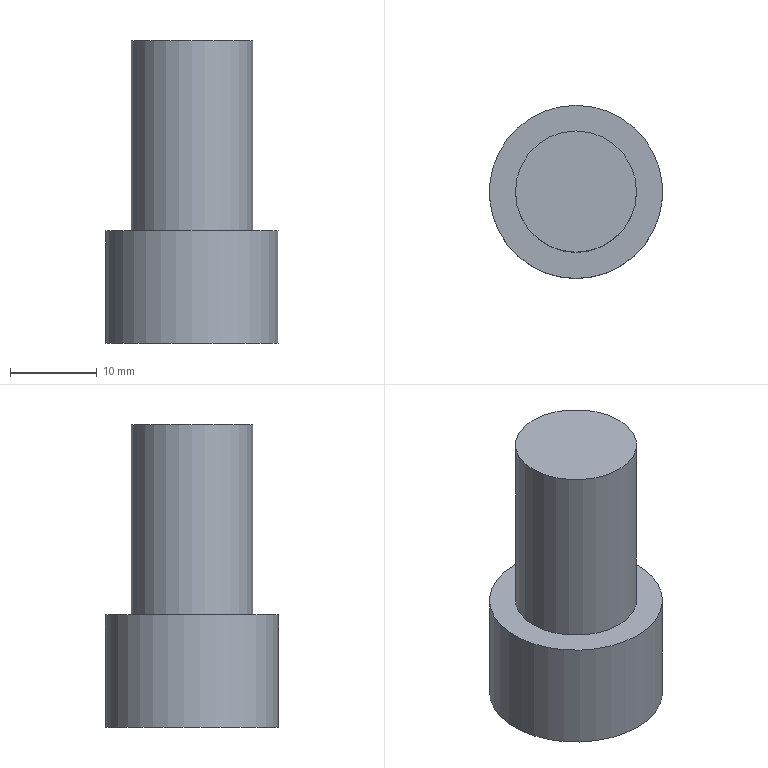Part | NX | features 模具.stp<1>[117] 2 | 1 solid | 5 faces | box 20 x 20 x 35 mm | volume 7471 mm3 | plane 3 | cylinder 2 | commonest cylinder face diameters 14 x1 20 x1
STEP:
#1=CARTESIAN_POINT('',(70.,110.,-285.5));
#2=VERTEX_POINT('',#1);
#3=CARTESIAN_POINT('',(70.,100.,-285.5));
#4=DIRECTION('',(0.,0.,1.));
#5=DIRECTION('',(0.,1.,0.));
#6=AXIS2_PLACEMENT_3D('',#3,#4,#5);
#7=CIRCLE('',#6,10.);
#8=EDGE_CURVE('',#2,#2,#7,.T.);
#9=ORIENTED_EDGE('',*,*,#8,.F.);
#10=EDGE_LOOP('',(#9));
#11=FACE_BOUND('',#10,.T.);
#12=CARTESIAN_POINT('',(70.,100.,-285.5));
#13=DIRECTION('',(0.,0.,-1.));
#14=DIRECTION('',(0.,-1.,0.));
#15=AXIS2_PLACEMENT_3D('',#12,#13,#14);
#16=PLANE('',#15);
#17=ADVANCED_FACE('',(#11),#16,.T.);
#18=CARTESIAN_POINT('',(70.,110.,-272.5));
#19=VERTEX_POINT('',#18);
#20=CARTESIAN_POINT('',(70.,100.,-272.5));
#21=DIRECTION('',(0.,0.,-1.));
#22=DIRECTION('',(0.,1.,0.));
#23=AXIS2_PLACEMENT_3D('',#20,#21,#22);
#24=CIRCLE('',#23,10.);
#25=EDGE_CURVE('',#19,#19,#24,.T.);
#26=ORIENTED_EDGE('',*,*,#25,.T.);
#27=EDGE_LOOP('',(#26));
#28=FACE_BOUND('',#27,.T.);
#29=ORIENTED_EDGE('',*,*,#8,.T.);
#30=EDGE_LOOP('',(#29));
#31=FACE_BOUND('',#30,.T.);
#32=CARTESIAN_POINT('',(70.,100.,-272.5));
#33=DIRECTION('',(0.,0.,-1.));
#34=DIRECTION('',(0.,1.,0.));
#35=AXIS2_PLACEMENT_3D('',#32,#33,#34);
#36=CYLINDRICAL_SURFACE('',#35,10.);
#37=ADVANCED_FACE('',(#28,#31),#36,.T.);
#38=ORIENTED_EDGE('',*,*,#25,.F.);
#39=EDGE_LOOP('',(#38));
#40=FACE_BOUND('',#39,.T.);
#41=CARTESIAN_POINT('',(70.,93.,-272.5));
#42=VERTEX_POINT('',#41);
#43=CARTESIAN_POINT('',(70.,100.,-272.5));
#44=DIRECTION('',(0.,0.,-1.));
#45=DIRECTION('',(0.,-1.,0.));
#46=AXIS2_PLACEMENT_3D('',#43,#44,#45);
#47=CIRCLE('',#46,7.);
#48=EDGE_CURVE('',#42,#42,#47,.T.);
#49=ORIENTED_EDGE('',*,*,#48,.T.);
#50=EDGE_LOOP('',(#49));
#51=FACE_BOUND('',#50,.T.);
#52=CARTESIAN_POINT('',(70.,100.,-272.5));
#53=DIRECTION('',(0.,0.,1.));
#54=DIRECTION('',(0.,-1.,0.));
#55=AXIS2_PLACEMENT_3D('',#52,#53,#54);
#56=PLANE('',#55);
#57=ADVANCED_FACE('',(#40,#51),#56,.T.);
#58=CARTESIAN_POINT('',(70.,107.,-250.5));
#59=VERTEX_POINT('',#58);
#60=CARTESIAN_POINT('',(70.,100.,-250.5));
#61=DIRECTION('',(0.,0.,-1.));
#62=DIRECTION('',(0.,1.,0.));
#63=AXIS2_PLACEMENT_3D('',#60,#61,#62);
#64=CIRCLE('',#63,7.);
#65=EDGE_CURVE('',#59,#59,#64,.T.);
#66=ORIENTED_EDGE('',*,*,#65,.T.);
#67=EDGE_LOOP('',(#66));
#68=FACE_BOUND('',#67,.T.);
#69=ORIENTED_EDGE('',*,*,#48,.F.);
#70=EDGE_LOOP('',(#69));
#71=FACE_BOUND('',#70,.T.);
#72=CARTESIAN_POINT('',(70.,100.,-250.5));
#73=DIRECTION('',(0.,0.,-1.));
#74=DIRECTION('',(0.,1.,0.));
#75=AXIS2_PLACEMENT_3D('',#72,#73,#74);
#76=CYLINDRICAL_SURFACE('',#75,7.);
#77=ADVANCED_FACE('',(#68,#71),#76,.T.);
#78=ORIENTED_EDGE('',*,*,#65,.F.);
#79=EDGE_LOOP('',(#78));
#80=FACE_BOUND('',#79,.T.);
#81=CARTESIAN_POINT('',(70.,100.,-250.5));
#82=DIRECTION('',(0.,0.,1.));
#83=DIRECTION('',(0.,-1.,0.));
#84=AXIS2_PLACEMENT_3D('',#81,#82,#83);
#85=PLANE('',#84);
#86=ADVANCED_FACE('',(#80),#85,.T.);
#87=CLOSED_SHELL('',(#17,#37,#57,#77,#86));
#88=MANIFOLD_SOLID_BREP('',#87);
#89=(LENGTH_UNIT()NAMED_UNIT(*)SI_UNIT(.MILLI.,.METRE.));
#90=UNCERTAINTY_MEASURE_WITH_UNIT(LENGTH_MEASURE(0.00001),#89,'','');
#91=(NAMED_UNIT(*)PLANE_ANGLE_UNIT()SI_UNIT($,.RADIAN.));
#92=(NAMED_UNIT(*)SI_UNIT($,.STERADIAN.)SOLID_ANGLE_UNIT());
#93=(GEOMETRIC_REPRESENTATION_CONTEXT(3)GLOBAL_UNCERTAINTY_ASSIGNED_CONTEXT((#90))GLOBAL_UNIT_ASSIGNED_CONTEXT((#89,#91,#92))REPRESENTATION_CONTEXT('',''));
#94=ADVANCED_BREP_SHAPE_REPRESENTATION('',(#88),#93);